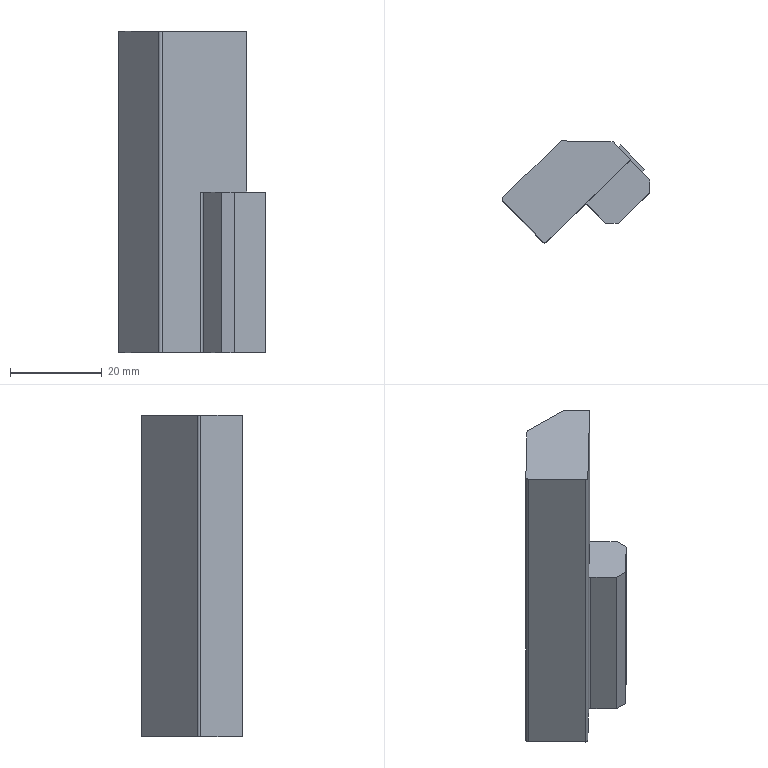Part | STEP file | gslz 2016.10.28-13_id1658_x_t | 1 solid | 19 faces | box 32.149 x 22.13 x 70 mm | volume 26166 mm3 | plane 15 | cylinder 3 | other 1 | commonest cylinder face diameters 1 x3